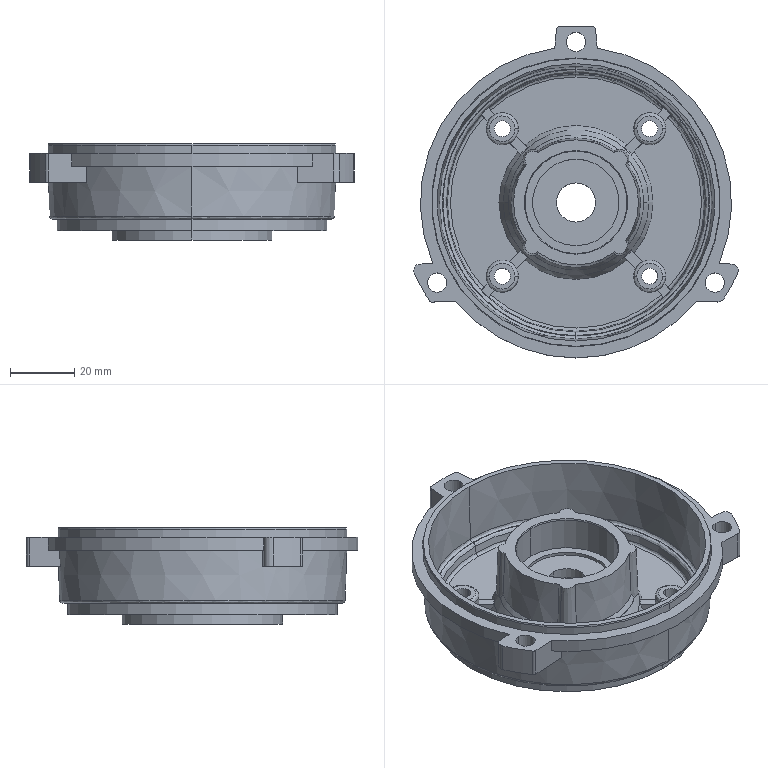Part | SolidWorks | features BaseBody 1 | 1 solid | 195 faces | box 101.12 x 103.5 x 30 mm | volume 47636 mm3 | plane 80 | cylinder 55 | cone 41 | spline 19 | commonest cylinder face diameters 5 x8 10 x8 6 x6 4 x4 2 x3 97 x3